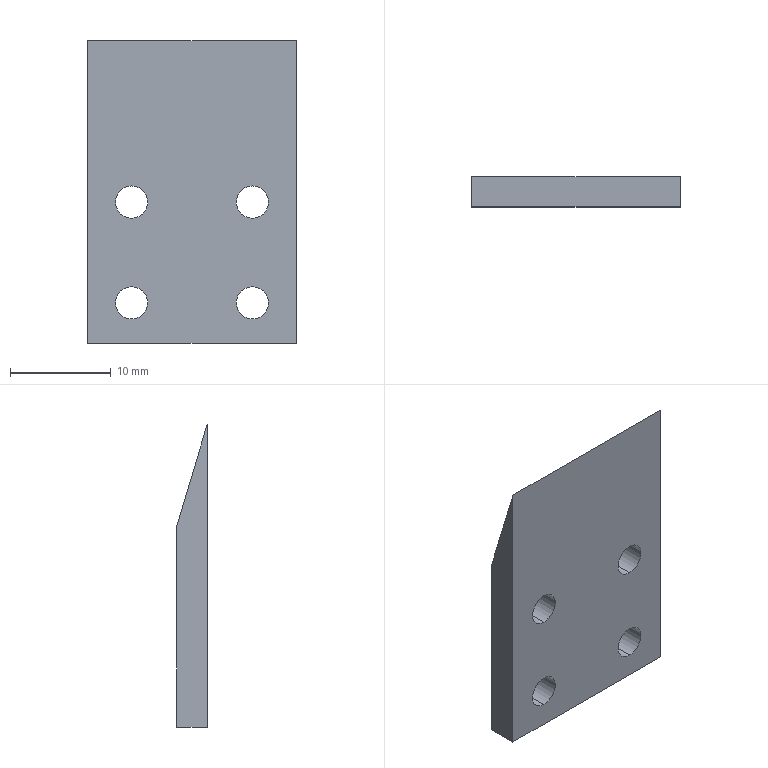Part | STEP file | Blade | 1 solid | 14 faces | box 20.7 x 3 x 30 mm | volume 1456 mm3 | cylinder 8 | plane 6 | commonest cylinder face diameters 3.2 x8
STEP:
#1=CARTESIAN_POINT('',(-6.,1.5,12.4));
#2=VERTEX_POINT('',#1);
#3=CARTESIAN_POINT('',(-6.,1.5,15.6));
#4=VERTEX_POINT('',#3);
#5=CARTESIAN_POINT('',(-6.,1.5,14.));
#6=DIRECTION('',(0.,1.,0.));
#7=DIRECTION('',(0.,0.,-1.));
#8=AXIS2_PLACEMENT_3D('',#5,#6,#7);
#9=CIRCLE('',#8,1.6);
#10=EDGE_CURVE('',#2,#4,#9,.T.);
#11=ORIENTED_EDGE('',*,*,#10,.T.);
#12=CARTESIAN_POINT('',(-6.,-1.5,15.6));
#13=VERTEX_POINT('',#12);
#14=CARTESIAN_POINT('',(-6.,38.5,15.6));
#15=DIRECTION('',(0.,-1.,0.));
#16=VECTOR('',#15,1000.);
#17=LINE('',#14,#16);
#18=EDGE_CURVE('',#4,#13,#17,.T.);
#19=ORIENTED_EDGE('',*,*,#18,.T.);
#20=CARTESIAN_POINT('',(-6.,-1.5,12.4));
#21=VERTEX_POINT('',#20);
#22=CARTESIAN_POINT('',(-6.,-1.5,14.));
#23=DIRECTION('',(0.,1.,0.));
#24=DIRECTION('',(0.,0.,-1.));
#25=AXIS2_PLACEMENT_3D('',#22,#23,#24);
#26=CIRCLE('',#25,1.6);
#27=EDGE_CURVE('',#21,#13,#26,.T.);
#28=ORIENTED_EDGE('',*,*,#27,.F.);
#29=CARTESIAN_POINT('',(-6.,38.5,12.4));
#30=DIRECTION('',(0.,-1.,0.));
#31=VECTOR('',#30,1000.);
#32=LINE('',#29,#31);
#33=EDGE_CURVE('',#2,#21,#32,.T.);
#34=ORIENTED_EDGE('',*,*,#33,.F.);
#35=EDGE_LOOP('',(#11,#19,#28,#34));
#36=FACE_OUTER_BOUND('',#35,.T.);
#37=CARTESIAN_POINT('',(-6.,38.5,14.));
#38=DIRECTION('',(0.,-1.,0.));
#39=DIRECTION('',(0.,0.,-1.));
#40=AXIS2_PLACEMENT_3D('',#37,#38,#39);
#41=CYLINDRICAL_SURFACE('',#40,1.6);
#42=ADVANCED_FACE('',(#36),#41,.F.);
#43=CARTESIAN_POINT('',(-6.,1.5,2.4));
#44=VERTEX_POINT('',#43);
#45=CARTESIAN_POINT('',(-6.,1.5,5.6));
#46=VERTEX_POINT('',#45);
#47=CARTESIAN_POINT('',(-6.,1.5,4.));
#48=DIRECTION('',(0.,1.,0.));
#49=DIRECTION('',(0.,0.,-1.));
#50=AXIS2_PLACEMENT_3D('',#47,#48,#49);
#51=CIRCLE('',#50,1.6);
#52=EDGE_CURVE('',#44,#46,#51,.T.);
#53=ORIENTED_EDGE('',*,*,#52,.T.);
#54=CARTESIAN_POINT('',(-6.,-1.5,5.6));
#55=VERTEX_POINT('',#54);
#56=CARTESIAN_POINT('',(-6.,38.5,5.6));
#57=DIRECTION('',(0.,-1.,0.));
#58=VECTOR('',#57,1000.);
#59=LINE('',#56,#58);
#60=EDGE_CURVE('',#46,#55,#59,.T.);
#61=ORIENTED_EDGE('',*,*,#60,.T.);
#62=CARTESIAN_POINT('',(-6.,-1.5,2.4));
#63=VERTEX_POINT('',#62);
#64=CARTESIAN_POINT('',(-6.,-1.5,4.));
#65=DIRECTION('',(0.,1.,0.));
#66=DIRECTION('',(0.,0.,-1.));
#67=AXIS2_PLACEMENT_3D('',#64,#65,#66);
#68=CIRCLE('',#67,1.6);
#69=EDGE_CURVE('',#63,#55,#68,.T.);
#70=ORIENTED_EDGE('',*,*,#69,.F.);
#71=CARTESIAN_POINT('',(-6.,38.5,2.4));
#72=DIRECTION('',(0.,-1.,0.));
#73=VECTOR('',#72,1000.);
#74=LINE('',#71,#73);
#75=EDGE_CURVE('',#44,#63,#74,.T.);
#76=ORIENTED_EDGE('',*,*,#75,.F.);
#77=EDGE_LOOP('',(#53,#61,#70,#76));
#78=FACE_OUTER_BOUND('',#77,.T.);
#79=CARTESIAN_POINT('',(-6.,38.5,4.));
#80=DIRECTION('',(0.,-1.,0.));
#81=DIRECTION('',(0.,0.,-1.));
#82=AXIS2_PLACEMENT_3D('',#79,#80,#81);
#83=CYLINDRICAL_SURFACE('',#82,1.6);
#84=ADVANCED_FACE('',(#78),#83,.F.);
#85=CARTESIAN_POINT('',(6.,1.5,15.6));
#86=VERTEX_POINT('',#85);
#87=CARTESIAN_POINT('',(6.,1.5,12.4));
#88=VERTEX_POINT('',#87);
#89=CARTESIAN_POINT('',(6.,1.5,14.));
#90=DIRECTION('',(0.,-1.,0.));
#91=DIRECTION('',(0.,0.,-1.));
#92=AXIS2_PLACEMENT_3D('',#89,#90,#91);
#93=CIRCLE('',#92,1.6);
#94=EDGE_CURVE('',#86,#88,#93,.T.);
#95=ORIENTED_EDGE('',*,*,#94,.F.);
#96=CARTESIAN_POINT('',(6.,-1.5,15.6));
#97=VERTEX_POINT('',#96);
#98=CARTESIAN_POINT('',(6.,38.5,15.6));
#99=DIRECTION('',(0.,-1.,0.));
#100=VECTOR('',#99,1000.);
#101=LINE('',#98,#100);
#102=EDGE_CURVE('',#86,#97,#101,.T.);
#103=ORIENTED_EDGE('',*,*,#102,.T.);
#104=CARTESIAN_POINT('',(6.,-1.5,12.4));
#105=VERTEX_POINT('',#104);
#106=CARTESIAN_POINT('',(6.,-1.5,14.));
#107=DIRECTION('',(0.,-1.,0.));
#108=DIRECTION('',(0.,0.,-1.));
#109=AXIS2_PLACEMENT_3D('',#106,#107,#108);
#110=CIRCLE('',#109,1.6);
#111=EDGE_CURVE('',#97,#105,#110,.T.);
#112=ORIENTED_EDGE('',*,*,#111,.T.);
#113=CARTESIAN_POINT('',(6.,38.5,12.4));
#114=DIRECTION('',(0.,-1.,0.));
#115=VECTOR('',#114,1000.);
#116=LINE('',#113,#115);
#117=EDGE_CURVE('',#88,#105,#116,.T.);
#118=ORIENTED_EDGE('',*,*,#117,.F.);
#119=EDGE_LOOP('',(#95,#103,#112,#118));
#120=FACE_OUTER_BOUND('',#119,.T.);
#121=CARTESIAN_POINT('',(6.,38.5,14.));
#122=DIRECTION('',(0.,-1.,0.));
#123=DIRECTION('',(0.,0.,-1.));
#124=AXIS2_PLACEMENT_3D('',#121,#122,#123);
#125=CYLINDRICAL_SURFACE('',#124,1.6);
#126=ADVANCED_FACE('',(#120),#125,.F.);
#127=CARTESIAN_POINT('',(6.,1.5,5.6));
#128=VERTEX_POINT('',#127);
#129=CARTESIAN_POINT('',(6.,1.5,2.4));
#130=VERTEX_POINT('',#129);
#131=CARTESIAN_POINT('',(6.,1.5,4.));
#132=DIRECTION('',(0.,-1.,0.));
#133=DIRECTION('',(0.,0.,-1.));
#134=AXIS2_PLACEMENT_3D('',#131,#132,#133);
#135=CIRCLE('',#134,1.6);
#136=EDGE_CURVE('',#128,#130,#135,.T.);
#137=ORIENTED_EDGE('',*,*,#136,.F.);
#138=CARTESIAN_POINT('',(6.,-1.5,5.6));
#139=VERTEX_POINT('',#138);
#140=CARTESIAN_POINT('',(6.,38.5,5.6));
#141=DIRECTION('',(0.,-1.,0.));
#142=VECTOR('',#141,1000.);
#143=LINE('',#140,#142);
#144=EDGE_CURVE('',#128,#139,#143,.T.);
#145=ORIENTED_EDGE('',*,*,#144,.T.);
#146=CARTESIAN_POINT('',(6.,-1.5,2.4));
#147=VERTEX_POINT('',#146);
#148=CARTESIAN_POINT('',(6.,-1.5,4.));
#149=DIRECTION('',(0.,-1.,0.));
#150=DIRECTION('',(0.,0.,-1.));
#151=AXIS2_PLACEMENT_3D('',#148,#149,#150);
#152=CIRCLE('',#151,1.6);
#153=EDGE_CURVE('',#139,#147,#152,.T.);
#154=ORIENTED_EDGE('',*,*,#153,.T.);
#155=CARTESIAN_POINT('',(6.,38.5,2.4));
#156=DIRECTION('',(0.,-1.,0.));
#157=VECTOR('',#156,1000.);
#158=LINE('',#155,#157);
#159=EDGE_CURVE('',#130,#147,#158,.T.);
#160=ORIENTED_EDGE('',*,*,#159,.F.);
#161=EDGE_LOOP('',(#137,#145,#154,#160));
#162=FACE_OUTER_BOUND('',#161,.T.);
#163=CARTESIAN_POINT('',(6.,38.5,4.));
#164=DIRECTION('',(0.,-1.,0.));
#165=DIRECTION('',(0.,0.,-1.));
#166=AXIS2_PLACEMENT_3D('',#163,#164,#165);
#167=CYLINDRICAL_SURFACE('',#166,1.6);
#168=ADVANCED_FACE('',(#162),#167,.F.);
#169=CARTESIAN_POINT('',(10.35,1.5,20.));
#170=VERTEX_POINT('',#169);
#171=CARTESIAN_POINT('',(10.35,1.5,0.));
#172=VERTEX_POINT('',#171);
#173=CARTESIAN_POINT('',(10.35,1.5,30.));
#174=DIRECTION('',(0.,0.,-1.));
#175=VECTOR('',#174,1000.);
#176=LINE('',#173,#175);
#177=EDGE_CURVE('',#170,#172,#176,.T.);
#178=ORIENTED_EDGE('',*,*,#177,.F.);
#179=CARTESIAN_POINT('',(10.35,-1.5,30.));
#180=VERTEX_POINT('',#179);
#181=CARTESIAN_POINT('',(10.35,-1.5,30.));
#182=DIRECTION('',(0.,0.2873,-0.9578));
#183=VECTOR('',#182,1000.);
#184=LINE('',#181,#183);
#185=EDGE_CURVE('',#180,#170,#184,.T.);
#186=ORIENTED_EDGE('',*,*,#185,.F.);
#187=CARTESIAN_POINT('',(10.35,-1.5,0.));
#188=VERTEX_POINT('',#187);
#189=CARTESIAN_POINT('',(10.35,-1.5,30.));
#190=DIRECTION('',(0.,0.,-1.));
#191=VECTOR('',#190,1000.);
#192=LINE('',#189,#191);
#193=EDGE_CURVE('',#180,#188,#192,.T.);
#194=ORIENTED_EDGE('',*,*,#193,.T.);
#195=CARTESIAN_POINT('',(10.35,1.5,0.));
#196=DIRECTION('',(0.,1.,0.));
#197=VECTOR('',#196,1000.);
#198=LINE('',#195,#197);
#199=EDGE_CURVE('',#188,#172,#198,.T.);
#200=ORIENTED_EDGE('',*,*,#199,.T.);
#201=EDGE_LOOP('',(#178,#186,#194,#200));
#202=FACE_OUTER_BOUND('',#201,.T.);
#203=CARTESIAN_POINT('',(10.35,1.5,30.));
#204=DIRECTION('',(-1.,0.,0.));
#205=DIRECTION('',(0.,0.,1.));
#206=AXIS2_PLACEMENT_3D('',#203,#204,#205);
#207=PLANE('',#206);
#208=ADVANCED_FACE('',(#202),#207,.F.);
#209=ORIENTED_EDGE('',*,*,#10,.F.);
#210=CARTESIAN_POINT('',(-6.,1.5,14.));
#211=DIRECTION('',(0.,1.,0.));
#212=DIRECTION('',(0.,0.,-1.));
#213=AXIS2_PLACEMENT_3D('',#210,#211,#212);
#214=CIRCLE('',#213,1.6);
#215=EDGE_CURVE('',#4,#2,#214,.T.);
#216=ORIENTED_EDGE('',*,*,#215,.F.);
#217=EDGE_LOOP('',(#209,#216));
#218=FACE_BOUND('',#217,.T.);
#219=ORIENTED_EDGE('',*,*,#52,.F.);
#220=CARTESIAN_POINT('',(-6.,1.5,4.));
#221=DIRECTION('',(0.,1.,0.));
#222=DIRECTION('',(0.,0.,-1.));
#223=AXIS2_PLACEMENT_3D('',#220,#221,#222);
#224=CIRCLE('',#223,1.6);
#225=EDGE_CURVE('',#46,#44,#224,.T.);
#226=ORIENTED_EDGE('',*,*,#225,.F.);
#227=EDGE_LOOP('',(#219,#226));
#228=FACE_BOUND('',#227,.T.);
#229=CARTESIAN_POINT('',(6.,1.5,14.));
#230=DIRECTION('',(0.,-1.,0.));
#231=DIRECTION('',(0.,0.,-1.));
#232=AXIS2_PLACEMENT_3D('',#229,#230,#231);
#233=CIRCLE('',#232,1.6);
#234=EDGE_CURVE('',#88,#86,#233,.T.);
#235=ORIENTED_EDGE('',*,*,#234,.T.);
#236=ORIENTED_EDGE('',*,*,#94,.T.);
#237=EDGE_LOOP('',(#235,#236));
#238=FACE_BOUND('',#237,.T.);
#239=CARTESIAN_POINT('',(6.,1.5,4.));
#240=DIRECTION('',(0.,-1.,0.));
#241=DIRECTION('',(0.,0.,-1.));
#242=AXIS2_PLACEMENT_3D('',#239,#240,#241);
#243=CIRCLE('',#242,1.6);
#244=EDGE_CURVE('',#130,#128,#243,.T.);
#245=ORIENTED_EDGE('',*,*,#244,.T.);
#246=ORIENTED_EDGE('',*,*,#136,.T.);
#247=EDGE_LOOP('',(#245,#246));
#248=FACE_BOUND('',#247,.T.);
#249=CARTESIAN_POINT('',(-10.35,1.5,20.));
#250=VERTEX_POINT('',#249);
#251=CARTESIAN_POINT('',(-10.35,1.5,0.));
#252=VERTEX_POINT('',#251);
#253=CARTESIAN_POINT('',(-10.35,1.5,30.));
#254=DIRECTION('',(0.,0.,-1.));
#255=VECTOR('',#254,1000.);
#256=LINE('',#253,#255);
#257=EDGE_CURVE('',#250,#252,#256,.T.);
#258=ORIENTED_EDGE('',*,*,#257,.F.);
#259=CARTESIAN_POINT('',(-19.65,1.5,20.));
#260=DIRECTION('',(1.,0.,0.));
#261=VECTOR('',#260,1000.);
#262=LINE('',#259,#261);
#263=EDGE_CURVE('',#250,#170,#262,.T.);
#264=ORIENTED_EDGE('',*,*,#263,.T.);
#265=ORIENTED_EDGE('',*,*,#177,.T.);
#266=CARTESIAN_POINT('',(-10.35,1.5,0.));
#267=DIRECTION('',(-1.,0.,0.));
#268=VECTOR('',#267,1000.);
#269=LINE('',#266,#268);
#270=EDGE_CURVE('',#172,#252,#269,.T.);
#271=ORIENTED_EDGE('',*,*,#270,.T.);
#272=EDGE_LOOP('',(#258,#264,#265,#271));
#273=FACE_OUTER_BOUND('',#272,.T.);
#274=CARTESIAN_POINT('',(-10.35,1.5,30.));
#275=DIRECTION('',(0.,-1.,0.));
#276=DIRECTION('',(0.,0.,-1.));
#277=AXIS2_PLACEMENT_3D('',#274,#275,#276);
#278=PLANE('',#277);
#279=ADVANCED_FACE('',(#218,#228,#238,#248,#273),#278,.F.);
#280=CARTESIAN_POINT('',(-10.35,-1.5,30.));
#281=VERTEX_POINT('',#280);
#282=CARTESIAN_POINT('',(-10.35,-1.5,0.));
#283=VERTEX_POINT('',#282);
#284=CARTESIAN_POINT('',(-10.35,-1.5,30.));
#285=DIRECTION('',(0.,0.,-1.));
#286=VECTOR('',#285,1000.);
#287=LINE('',#284,#286);
#288=EDGE_CURVE('',#281,#283,#287,.T.);
#289=ORIENTED_EDGE('',*,*,#288,.F.);
#290=CARTESIAN_POINT('',(-10.35,-1.252,29.174));
#291=DIRECTION('',(0.,0.2873,-0.9578));
#292=VECTOR('',#291,1000.);
#293=LINE('',#290,#292);
#294=EDGE_CURVE('',#281,#250,#293,.T.);
#295=ORIENTED_EDGE('',*,*,#294,.T.);
#296=ORIENTED_EDGE('',*,*,#257,.T.);
#297=CARTESIAN_POINT('',(-10.35,1.5,0.));
#298=DIRECTION('',(0.,-1.,0.));
#299=VECTOR('',#298,1000.);
#300=LINE('',#297,#299);
#301=EDGE_CURVE('',#252,#283,#300,.T.);
#302=ORIENTED_EDGE('',*,*,#301,.T.);
#303=EDGE_LOOP('',(#289,#295,#296,#302));
#304=FACE_OUTER_BOUND('',#303,.T.);
#305=CARTESIAN_POINT('',(-10.35,1.5,30.));
#306=DIRECTION('',(1.,0.,0.));
#307=DIRECTION('',(0.,0.,-1.));
#308=AXIS2_PLACEMENT_3D('',#305,#306,#307);
#309=PLANE('',#308);
#310=ADVANCED_FACE('',(#304),#309,.F.);
#311=ORIENTED_EDGE('',*,*,#27,.T.);
#312=CARTESIAN_POINT('',(-6.,-1.5,14.));
#313=DIRECTION('',(0.,1.,0.));
#314=DIRECTION('',(0.,0.,-1.));
#315=AXIS2_PLACEMENT_3D('',#312,#313,#314);
#316=CIRCLE('',#315,1.6);
#317=EDGE_CURVE('',#13,#21,#316,.T.);
#318=ORIENTED_EDGE('',*,*,#317,.T.);
#319=EDGE_LOOP('',(#311,#318));
#320=FACE_BOUND('',#319,.T.);
#321=ORIENTED_EDGE('',*,*,#69,.T.);
#322=CARTESIAN_POINT('',(-6.,-1.5,4.));
#323=DIRECTION('',(0.,1.,0.));
#324=DIRECTION('',(0.,0.,-1.));
#325=AXIS2_PLACEMENT_3D('',#322,#323,#324);
#326=CIRCLE('',#325,1.6);
#327=EDGE_CURVE('',#55,#63,#326,.T.);
#328=ORIENTED_EDGE('',*,*,#327,.T.);
#329=EDGE_LOOP('',(#321,#328));
#330=FACE_BOUND('',#329,.T.);
#331=CARTESIAN_POINT('',(6.,-1.5,14.));
#332=DIRECTION('',(0.,-1.,0.));
#333=DIRECTION('',(0.,0.,-1.));
#334=AXIS2_PLACEMENT_3D('',#331,#332,#333);
#335=CIRCLE('',#334,1.6);
#336=EDGE_CURVE('',#105,#97,#335,.T.);
#337=ORIENTED_EDGE('',*,*,#336,.F.);
#338=ORIENTED_EDGE('',*,*,#111,.F.);
#339=EDGE_LOOP('',(#337,#338));
#340=FACE_BOUND('',#339,.T.);
#341=CARTESIAN_POINT('',(6.,-1.5,4.));
#342=DIRECTION('',(0.,-1.,0.));
#343=DIRECTION('',(0.,0.,-1.));
#344=AXIS2_PLACEMENT_3D('',#341,#342,#343);
#345=CIRCLE('',#344,1.6);
#346=EDGE_CURVE('',#147,#139,#345,.T.);
#347=ORIENTED_EDGE('',*,*,#346,.F.);
#348=ORIENTED_EDGE('',*,*,#153,.F.);
#349=EDGE_LOOP('',(#347,#348));
#350=FACE_BOUND('',#349,.T.);
#351=CARTESIAN_POINT('',(-10.35,-1.5,0.));
#352=DIRECTION('',(1.,0.,0.));
#353=VECTOR('',#352,1000.);
#354=LINE('',#351,#353);
#355=EDGE_CURVE('',#283,#188,#354,.T.);
#356=ORIENTED_EDGE('',*,*,#355,.T.);
#357=ORIENTED_EDGE('',*,*,#193,.F.);
#358=CARTESIAN_POINT('',(-10.35,-1.5,30.));
#359=DIRECTION('',(1.,0.,0.));
#360=VECTOR('',#359,1000.);
#361=LINE('',#358,#360);
#362=EDGE_CURVE('',#281,#180,#361,.T.);
#363=ORIENTED_EDGE('',*,*,#362,.F.);
#364=ORIENTED_EDGE('',*,*,#288,.T.);
#365=EDGE_LOOP('',(#356,#357,#363,#364));
#366=FACE_OUTER_BOUND('',#365,.T.);
#367=CARTESIAN_POINT('',(-10.35,-1.5,30.));
#368=DIRECTION('',(0.,1.,0.));
#369=DIRECTION('',(0.,0.,1.));
#370=AXIS2_PLACEMENT_3D('',#367,#368,#369);
#371=PLANE('',#370);
#372=ADVANCED_FACE('',(#320,#330,#340,#350,#366),#371,.F.);
#373=ORIENTED_EDGE('',*,*,#199,.F.);
#374=ORIENTED_EDGE('',*,*,#355,.F.);
#375=ORIENTED_EDGE('',*,*,#301,.F.);
#376=ORIENTED_EDGE('',*,*,#270,.F.);
#377=EDGE_LOOP('',(#373,#374,#375,#376));
#378=FACE_OUTER_BOUND('',#377,.T.);
#379=CARTESIAN_POINT('',(0.,0.,0.));
#380=DIRECTION('',(0.,0.,1.));
#381=DIRECTION('',(1.,0.,0.));
#382=AXIS2_PLACEMENT_3D('',#379,#380,#381);
#383=PLANE('',#382);
#384=ADVANCED_FACE('',(#378),#383,.F.);
#385=ORIENTED_EDGE('',*,*,#144,.F.);
#386=ORIENTED_EDGE('',*,*,#244,.F.);
#387=ORIENTED_EDGE('',*,*,#159,.T.);
#388=ORIENTED_EDGE('',*,*,#346,.T.);
#389=EDGE_LOOP('',(#385,#386,#387,#388));
#390=FACE_OUTER_BOUND('',#389,.T.);
#391=CARTESIAN_POINT('',(6.,38.5,4.));
#392=DIRECTION('',(0.,-1.,0.));
#393=DIRECTION('',(0.,0.,-1.));
#394=AXIS2_PLACEMENT_3D('',#391,#392,#393);
#395=CYLINDRICAL_SURFACE('',#394,1.6);
#396=ADVANCED_FACE('',(#390),#395,.F.);
#397=ORIENTED_EDGE('',*,*,#102,.F.);
#398=ORIENTED_EDGE('',*,*,#234,.F.);
#399=ORIENTED_EDGE('',*,*,#117,.T.);
#400=ORIENTED_EDGE('',*,*,#336,.T.);
#401=EDGE_LOOP('',(#397,#398,#399,#400));
#402=FACE_OUTER_BOUND('',#401,.T.);
#403=CARTESIAN_POINT('',(6.,38.5,14.));
#404=DIRECTION('',(0.,-1.,0.));
#405=DIRECTION('',(0.,0.,-1.));
#406=AXIS2_PLACEMENT_3D('',#403,#404,#405);
#407=CYLINDRICAL_SURFACE('',#406,1.6);
#408=ADVANCED_FACE('',(#402),#407,.F.);
#409=ORIENTED_EDGE('',*,*,#60,.F.);
#410=ORIENTED_EDGE('',*,*,#225,.T.);
#411=ORIENTED_EDGE('',*,*,#75,.T.);
#412=ORIENTED_EDGE('',*,*,#327,.F.);
#413=EDGE_LOOP('',(#409,#410,#411,#412));
#414=FACE_OUTER_BOUND('',#413,.T.);
#415=CARTESIAN_POINT('',(-6.,38.5,4.));
#416=DIRECTION('',(0.,-1.,0.));
#417=DIRECTION('',(0.,0.,-1.));
#418=AXIS2_PLACEMENT_3D('',#415,#416,#417);
#419=CYLINDRICAL_SURFACE('',#418,1.6);
#420=ADVANCED_FACE('',(#414),#419,.F.);
#421=ORIENTED_EDGE('',*,*,#18,.F.);
#422=ORIENTED_EDGE('',*,*,#215,.T.);
#423=ORIENTED_EDGE('',*,*,#33,.T.);
#424=ORIENTED_EDGE('',*,*,#317,.F.);
#425=EDGE_LOOP('',(#421,#422,#423,#424));
#426=FACE_OUTER_BOUND('',#425,.T.);
#427=CARTESIAN_POINT('',(-6.,38.5,14.));
#428=DIRECTION('',(0.,-1.,0.));
#429=DIRECTION('',(0.,0.,-1.));
#430=AXIS2_PLACEMENT_3D('',#427,#428,#429);
#431=CYLINDRICAL_SURFACE('',#430,1.6);
#432=ADVANCED_FACE('',(#426),#431,.F.);
#433=ORIENTED_EDGE('',*,*,#362,.T.);
#434=ORIENTED_EDGE('',*,*,#185,.T.);
#435=ORIENTED_EDGE('',*,*,#263,.F.);
#436=ORIENTED_EDGE('',*,*,#294,.F.);
#437=EDGE_LOOP('',(#433,#434,#435,#436));
#438=FACE_OUTER_BOUND('',#437,.T.);
#439=CARTESIAN_POINT('',(-19.65,-1.5,30.));
#440=DIRECTION('',(0.,-0.9578,-0.2873));
#441=DIRECTION('',(0.,0.2873,-0.9578));
#442=AXIS2_PLACEMENT_3D('',#439,#440,#441);
#443=PLANE('',#442);
#444=ADVANCED_FACE('',(#438),#443,.F.);
#445=CLOSED_SHELL('',(#42,#84,#126,#168,#208,#279,#310,#372,#384,#396,#408,#420,#432,#444));
#446=MANIFOLD_SOLID_BREP('',#445);
#447=CARTESIAN_POINT('',(0.,0.,0.));
#448=DIRECTION('',(0.,0.,1.));
#449=DIRECTION('',(1.,0.,0.));
#450=AXIS2_PLACEMENT_3D('',#447,#448,#449);
#451=(LENGTH_UNIT()NAMED_UNIT(*)SI_UNIT(.MILLI.,.METRE.));
#452=UNCERTAINTY_MEASURE_WITH_UNIT(LENGTH_MEASURE(0.00001),#451,'','');
#453=(NAMED_UNIT(*)PLANE_ANGLE_UNIT()SI_UNIT($,.RADIAN.));
#454=(NAMED_UNIT(*)SI_UNIT($,.STERADIAN.)SOLID_ANGLE_UNIT());
#455=(GEOMETRIC_REPRESENTATION_CONTEXT(3)GLOBAL_UNCERTAINTY_ASSIGNED_CONTEXT((#452))GLOBAL_UNIT_ASSIGNED_CONTEXT((#451,#453,#454))REPRESENTATION_CONTEXT('',''));
#456=ADVANCED_BREP_SHAPE_REPRESENTATION('',(#446,#450),#455);